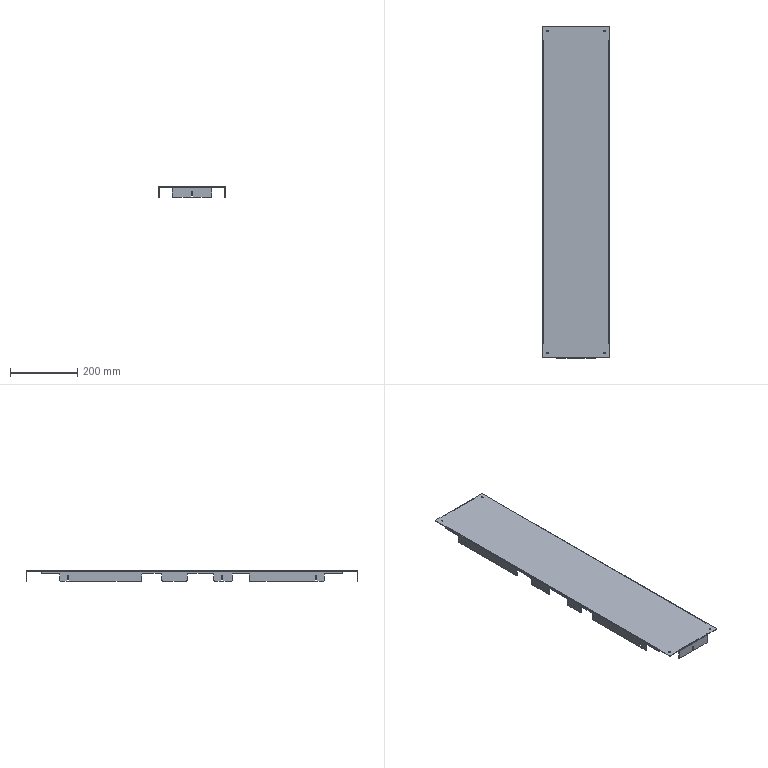Part | STEP file | 1 solid | 192 faces | box 199 x 989 x 30 mm | volume 288004 mm3 | plane 118 | cylinder 74 | commonest cylinder face diameters 4 x32 4.5 x14 10 x12 5 x8 1.2 x4 3.6 x4